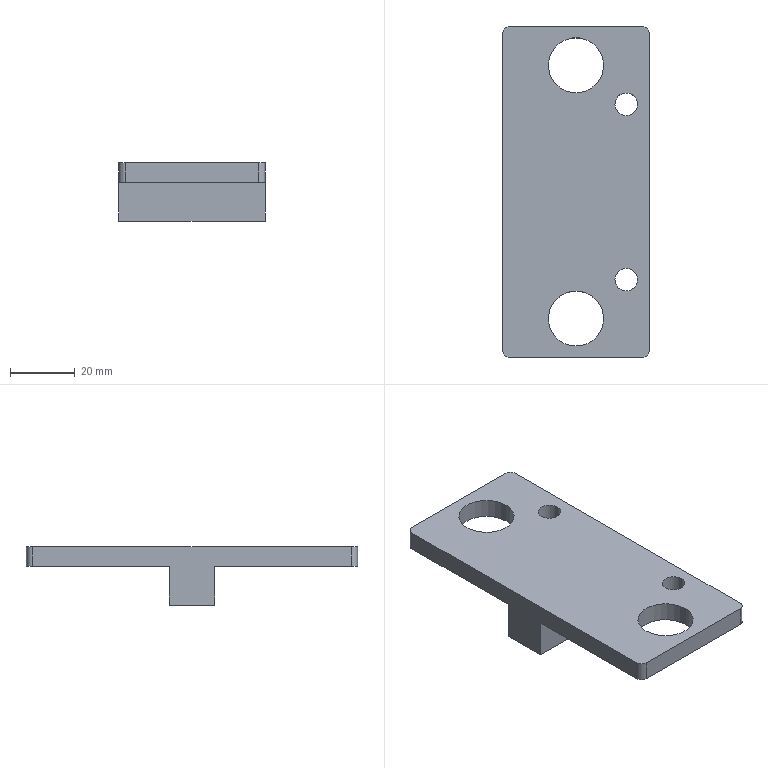Part | SolidWorks | features 3DProfileFeature 1, Extrusion 1, Fillet 1, HoleWzd 1, ICE 1, MirrorPattern 1 | 1 solid | 22 faces | box 45 x 102 x 18 mm | volume 31894 mm3 | cylinder 12 | plane 10 | commonest cylinder face diameters 4 x4 7 x4 17 x4
STEP:
#1=CARTESIAN_POINT('',(12.,-66.,0.));
#2=VERTEX_POINT('',#1);
#3=CARTESIAN_POINT('',(19.,-66.,0.));
#4=VERTEX_POINT('',#3);
#5=CARTESIAN_POINT('',(15.5,-66.,0.));
#6=DIRECTION('',(0.,0.,1.));
#7=DIRECTION('',(1.,0.,0.));
#8=AXIS2_PLACEMENT_3D('',#5,#6,#7);
#9=CIRCLE('',#8,3.5);
#10=EDGE_CURVE('',#2,#4,#9,.T.);
#11=ORIENTED_EDGE('',*,*,#10,.F.);
#12=CARTESIAN_POINT('',(12.,-66.,6.));
#13=VERTEX_POINT('',#12);
#14=CARTESIAN_POINT('',(12.,-66.,6.));
#15=DIRECTION('',(0.,0.,1.));
#16=VECTOR('',#15,1000.);
#17=LINE('',#14,#16);
#18=EDGE_CURVE('',#2,#13,#17,.T.);
#19=ORIENTED_EDGE('',*,*,#18,.T.);
#20=CARTESIAN_POINT('',(19.,-66.,6.));
#21=VERTEX_POINT('',#20);
#22=CARTESIAN_POINT('',(15.5,-66.,6.));
#23=DIRECTION('',(0.,0.,1.));
#24=DIRECTION('',(1.,0.,0.));
#25=AXIS2_PLACEMENT_3D('',#22,#23,#24);
#26=CIRCLE('',#25,3.5);
#27=EDGE_CURVE('',#13,#21,#26,.T.);
#28=ORIENTED_EDGE('',*,*,#27,.T.);
#29=CARTESIAN_POINT('',(19.,-66.,6.));
#30=DIRECTION('',(0.,0.,1.));
#31=VECTOR('',#30,1000.);
#32=LINE('',#29,#31);
#33=EDGE_CURVE('',#4,#21,#32,.T.);
#34=ORIENTED_EDGE('',*,*,#33,.F.);
#35=EDGE_LOOP('',(#11,#19,#28,#34));
#36=FACE_OUTER_BOUND('',#35,.T.);
#37=CARTESIAN_POINT('',(15.5,-66.,6.));
#38=DIRECTION('',(0.,0.,1.));
#39=DIRECTION('',(1.,0.,0.));
#40=AXIS2_PLACEMENT_3D('',#37,#38,#39);
#41=CYLINDRICAL_SURFACE('',#40,3.5);
#42=ADVANCED_FACE('',(#36),#41,.F.);
#43=CARTESIAN_POINT('',(8.5,-78.,6.));
#44=VERTEX_POINT('',#43);
#45=CARTESIAN_POINT('',(-8.5,-78.,6.));
#46=VERTEX_POINT('',#45);
#47=CARTESIAN_POINT('',(0.,-78.,6.));
#48=DIRECTION('',(0.,0.,-1.));
#49=DIRECTION('',(1.,0.,0.));
#50=AXIS2_PLACEMENT_3D('',#47,#48,#49);
#51=CIRCLE('',#50,8.5);
#52=EDGE_CURVE('',#44,#46,#51,.T.);
#53=ORIENTED_EDGE('',*,*,#52,.F.);
#54=CARTESIAN_POINT('',(8.5,-78.,0.));
#55=VERTEX_POINT('',#54);
#56=CARTESIAN_POINT('',(8.5,-78.,6.));
#57=DIRECTION('',(0.,0.,-1.));
#58=VECTOR('',#57,1000.);
#59=LINE('',#56,#58);
#60=EDGE_CURVE('',#44,#55,#59,.T.);
#61=ORIENTED_EDGE('',*,*,#60,.T.);
#62=CARTESIAN_POINT('',(-8.5,-78.,0.));
#63=VERTEX_POINT('',#62);
#64=CARTESIAN_POINT('',(0.,-78.,0.));
#65=DIRECTION('',(0.,0.,-1.));
#66=DIRECTION('',(1.,0.,0.));
#67=AXIS2_PLACEMENT_3D('',#64,#65,#66);
#68=CIRCLE('',#67,8.5);
#69=EDGE_CURVE('',#55,#63,#68,.T.);
#70=ORIENTED_EDGE('',*,*,#69,.T.);
#71=CARTESIAN_POINT('',(-8.5,-78.,6.));
#72=DIRECTION('',(0.,0.,-1.));
#73=VECTOR('',#72,1000.);
#74=LINE('',#71,#73);
#75=EDGE_CURVE('',#46,#63,#74,.T.);
#76=ORIENTED_EDGE('',*,*,#75,.F.);
#77=EDGE_LOOP('',(#53,#61,#70,#76));
#78=FACE_OUTER_BOUND('',#77,.T.);
#79=CARTESIAN_POINT('',(0.,-78.,6.));
#80=DIRECTION('',(0.,0.,-1.));
#81=DIRECTION('',(-1.,0.,0.));
#82=AXIS2_PLACEMENT_3D('',#79,#80,#81);
#83=CYLINDRICAL_SURFACE('',#82,8.5);
#84=ADVANCED_FACE('',(#78),#83,.F.);
#85=CARTESIAN_POINT('',(12.,-12.,0.));
#86=VERTEX_POINT('',#85);
#87=CARTESIAN_POINT('',(19.,-12.,0.));
#88=VERTEX_POINT('',#87);
#89=CARTESIAN_POINT('',(15.5,-12.,0.));
#90=DIRECTION('',(0.,0.,1.));
#91=DIRECTION('',(1.,0.,0.));
#92=AXIS2_PLACEMENT_3D('',#89,#90,#91);
#93=CIRCLE('',#92,3.5);
#94=EDGE_CURVE('',#86,#88,#93,.T.);
#95=ORIENTED_EDGE('',*,*,#94,.F.);
#96=CARTESIAN_POINT('',(12.,-12.,6.));
#97=VERTEX_POINT('',#96);
#98=CARTESIAN_POINT('',(12.,-12.,6.));
#99=DIRECTION('',(0.,0.,1.));
#100=VECTOR('',#99,1000.);
#101=LINE('',#98,#100);
#102=EDGE_CURVE('',#86,#97,#101,.T.);
#103=ORIENTED_EDGE('',*,*,#102,.T.);
#104=CARTESIAN_POINT('',(19.,-12.,6.));
#105=VERTEX_POINT('',#104);
#106=CARTESIAN_POINT('',(15.5,-12.,6.));
#107=DIRECTION('',(0.,0.,1.));
#108=DIRECTION('',(1.,0.,0.));
#109=AXIS2_PLACEMENT_3D('',#106,#107,#108);
#110=CIRCLE('',#109,3.5);
#111=EDGE_CURVE('',#97,#105,#110,.T.);
#112=ORIENTED_EDGE('',*,*,#111,.T.);
#113=CARTESIAN_POINT('',(19.,-12.,6.));
#114=DIRECTION('',(0.,0.,1.));
#115=VECTOR('',#114,1000.);
#116=LINE('',#113,#115);
#117=EDGE_CURVE('',#88,#105,#116,.T.);
#118=ORIENTED_EDGE('',*,*,#117,.F.);
#119=EDGE_LOOP('',(#95,#103,#112,#118));
#120=FACE_OUTER_BOUND('',#119,.T.);
#121=CARTESIAN_POINT('',(15.5,-12.,6.));
#122=DIRECTION('',(0.,0.,1.));
#123=DIRECTION('',(1.,0.,0.));
#124=AXIS2_PLACEMENT_3D('',#121,#122,#123);
#125=CYLINDRICAL_SURFACE('',#124,3.5);
#126=ADVANCED_FACE('',(#120),#125,.F.);
#127=CARTESIAN_POINT('',(-8.5,0.,6.));
#128=VERTEX_POINT('',#127);
#129=CARTESIAN_POINT('',(8.5,0.,6.));
#130=VERTEX_POINT('',#129);
#131=CARTESIAN_POINT('',(0.,0.,6.));
#132=DIRECTION('',(0.,0.,1.));
#133=DIRECTION('',(1.,0.,0.));
#134=AXIS2_PLACEMENT_3D('',#131,#132,#133);
#135=CIRCLE('',#134,8.5);
#136=EDGE_CURVE('',#128,#130,#135,.T.);
#137=ORIENTED_EDGE('',*,*,#136,.T.);
#138=CARTESIAN_POINT('',(8.5,0.,0.));
#139=VERTEX_POINT('',#138);
#140=CARTESIAN_POINT('',(8.5,0.,6.));
#141=DIRECTION('',(0.,0.,-1.));
#142=VECTOR('',#141,1000.);
#143=LINE('',#140,#142);
#144=EDGE_CURVE('',#130,#139,#143,.T.);
#145=ORIENTED_EDGE('',*,*,#144,.T.);
#146=CARTESIAN_POINT('',(-8.5,0.,0.));
#147=VERTEX_POINT('',#146);
#148=CARTESIAN_POINT('',(0.,0.,0.));
#149=DIRECTION('',(0.,0.,1.));
#150=DIRECTION('',(1.,0.,0.));
#151=AXIS2_PLACEMENT_3D('',#148,#149,#150);
#152=CIRCLE('',#151,8.5);
#153=EDGE_CURVE('',#147,#139,#152,.T.);
#154=ORIENTED_EDGE('',*,*,#153,.F.);
#155=CARTESIAN_POINT('',(-8.5,0.,6.));
#156=DIRECTION('',(0.,0.,-1.));
#157=VECTOR('',#156,1000.);
#158=LINE('',#155,#157);
#159=EDGE_CURVE('',#128,#147,#158,.T.);
#160=ORIENTED_EDGE('',*,*,#159,.F.);
#161=EDGE_LOOP('',(#137,#145,#154,#160));
#162=FACE_OUTER_BOUND('',#161,.T.);
#163=CARTESIAN_POINT('',(0.,0.,6.));
#164=DIRECTION('',(0.,0.,-1.));
#165=DIRECTION('',(-1.,0.,0.));
#166=AXIS2_PLACEMENT_3D('',#163,#164,#165);
#167=CYLINDRICAL_SURFACE('',#166,8.5);
#168=ADVANCED_FACE('',(#162),#167,.F.);
#169=CARTESIAN_POINT('',(-22.5,-46.,0.));
#170=VERTEX_POINT('',#169);
#171=CARTESIAN_POINT('',(22.5,-46.,0.));
#172=VERTEX_POINT('',#171);
#173=CARTESIAN_POINT('',(22.5,-46.,0.));
#174=DIRECTION('',(1.,0.,0.));
#175=VECTOR('',#174,1000.);
#176=LINE('',#173,#175);
#177=EDGE_CURVE('',#170,#172,#176,.T.);
#178=ORIENTED_EDGE('',*,*,#177,.F.);
#179=CARTESIAN_POINT('',(-22.5,-46.,-12.));
#180=VERTEX_POINT('',#179);
#181=CARTESIAN_POINT('',(-22.5,-46.,6.));
#182=DIRECTION('',(0.,0.,-1.));
#183=VECTOR('',#182,1000.);
#184=LINE('',#181,#183);
#185=EDGE_CURVE('',#170,#180,#184,.T.);
#186=ORIENTED_EDGE('',*,*,#185,.T.);
#187=CARTESIAN_POINT('',(22.5,-46.,-12.));
#188=VERTEX_POINT('',#187);
#189=CARTESIAN_POINT('',(22.5,-46.,-12.));
#190=DIRECTION('',(-1.,0.,0.));
#191=VECTOR('',#190,1000.);
#192=LINE('',#189,#191);
#193=EDGE_CURVE('',#188,#180,#192,.T.);
#194=ORIENTED_EDGE('',*,*,#193,.F.);
#195=CARTESIAN_POINT('',(22.5,-46.,6.));
#196=DIRECTION('',(0.,0.,-1.));
#197=VECTOR('',#196,1000.);
#198=LINE('',#195,#197);
#199=EDGE_CURVE('',#172,#188,#198,.T.);
#200=ORIENTED_EDGE('',*,*,#199,.F.);
#201=EDGE_LOOP('',(#178,#186,#194,#200));
#202=FACE_OUTER_BOUND('',#201,.T.);
#203=CARTESIAN_POINT('',(22.5,-46.,6.));
#204=DIRECTION('',(0.,1.,0.));
#205=DIRECTION('',(0.,0.,1.));
#206=AXIS2_PLACEMENT_3D('',#203,#204,#205);
#207=PLANE('',#206);
#208=ADVANCED_FACE('',(#202),#207,.F.);
#209=CARTESIAN_POINT('',(15.5,-12.,0.));
#210=DIRECTION('',(0.,0.,1.));
#211=DIRECTION('',(1.,0.,0.));
#212=AXIS2_PLACEMENT_3D('',#209,#210,#211);
#213=CIRCLE('',#212,3.5);
#214=EDGE_CURVE('',#88,#86,#213,.T.);
#215=ORIENTED_EDGE('',*,*,#214,.T.);
#216=ORIENTED_EDGE('',*,*,#94,.T.);
#217=EDGE_LOOP('',(#215,#216));
#218=FACE_BOUND('',#217,.T.);
#219=ORIENTED_EDGE('',*,*,#153,.T.);
#220=CARTESIAN_POINT('',(0.,0.,0.));
#221=DIRECTION('',(0.,0.,1.));
#222=DIRECTION('',(1.,0.,0.));
#223=AXIS2_PLACEMENT_3D('',#220,#221,#222);
#224=CIRCLE('',#223,8.5);
#225=EDGE_CURVE('',#139,#147,#224,.T.);
#226=ORIENTED_EDGE('',*,*,#225,.T.);
#227=EDGE_LOOP('',(#219,#226));
#228=FACE_BOUND('',#227,.T.);
#229=CARTESIAN_POINT('',(-22.5,10.,0.));
#230=VERTEX_POINT('',#229);
#231=CARTESIAN_POINT('',(-22.5,-32.,0.));
#232=VERTEX_POINT('',#231);
#233=CARTESIAN_POINT('',(-22.5,-46.,0.));
#234=DIRECTION('',(0.,-1.,0.));
#235=VECTOR('',#234,1000.);
#236=LINE('',#233,#235);
#237=EDGE_CURVE('',#230,#232,#236,.T.);
#238=ORIENTED_EDGE('',*,*,#237,.F.);
#239=CARTESIAN_POINT('',(-20.5,12.,0.));
#240=VERTEX_POINT('',#239);
#241=CARTESIAN_POINT('',(-20.5,10.,0.));
#242=DIRECTION('',(0.,0.,-1.));
#243=DIRECTION('',(1.,0.,0.));
#244=AXIS2_PLACEMENT_3D('',#241,#242,#243);
#245=CIRCLE('',#244,2.);
#246=EDGE_CURVE('',#230,#240,#245,.T.);
#247=ORIENTED_EDGE('',*,*,#246,.T.);
#248=CARTESIAN_POINT('',(20.5,12.,0.));
#249=VERTEX_POINT('',#248);
#250=CARTESIAN_POINT('',(22.5,12.,0.));
#251=DIRECTION('',(-1.,0.,0.));
#252=VECTOR('',#251,1000.);
#253=LINE('',#250,#252);
#254=EDGE_CURVE('',#249,#240,#253,.T.);
#255=ORIENTED_EDGE('',*,*,#254,.F.);
#256=CARTESIAN_POINT('',(22.5,10.,0.));
#257=VERTEX_POINT('',#256);
#258=CARTESIAN_POINT('',(20.5,10.,0.));
#259=DIRECTION('',(0.,0.,-1.));
#260=DIRECTION('',(1.,0.,0.));
#261=AXIS2_PLACEMENT_3D('',#258,#259,#260);
#262=CIRCLE('',#261,2.);
#263=EDGE_CURVE('',#249,#257,#262,.T.);
#264=ORIENTED_EDGE('',*,*,#263,.T.);
#265=CARTESIAN_POINT('',(22.5,-32.,0.));
#266=VERTEX_POINT('',#265);
#267=CARTESIAN_POINT('',(22.5,-46.,0.));
#268=DIRECTION('',(0.,1.,0.));
#269=VECTOR('',#268,1000.);
#270=LINE('',#267,#269);
#271=EDGE_CURVE('',#266,#257,#270,.T.);
#272=ORIENTED_EDGE('',*,*,#271,.F.);
#273=CARTESIAN_POINT('',(22.5,-32.,0.));
#274=DIRECTION('',(1.,0.,0.));
#275=VECTOR('',#274,1000.);
#276=LINE('',#273,#275);
#277=EDGE_CURVE('',#232,#266,#276,.T.);
#278=ORIENTED_EDGE('',*,*,#277,.F.);
#279=EDGE_LOOP('',(#238,#247,#255,#264,#272,#278));
#280=FACE_OUTER_BOUND('',#279,.T.);
#281=CARTESIAN_POINT('',(0.,0.,0.));
#282=DIRECTION('',(0.,0.,1.));
#283=DIRECTION('',(1.,0.,0.));
#284=AXIS2_PLACEMENT_3D('',#281,#282,#283);
#285=PLANE('',#284);
#286=ADVANCED_FACE('',(#218,#228,#280),#285,.F.);
#287=CARTESIAN_POINT('',(15.5,-66.,6.));
#288=DIRECTION('',(0.,0.,1.));
#289=DIRECTION('',(1.,0.,0.));
#290=AXIS2_PLACEMENT_3D('',#287,#288,#289);
#291=CIRCLE('',#290,3.5);
#292=EDGE_CURVE('',#21,#13,#291,.T.);
#293=ORIENTED_EDGE('',*,*,#292,.F.);
#294=ORIENTED_EDGE('',*,*,#27,.F.);
#295=EDGE_LOOP('',(#293,#294));
#296=FACE_BOUND('',#295,.T.);
#297=CARTESIAN_POINT('',(20.5,-90.,6.));
#298=VERTEX_POINT('',#297);
#299=CARTESIAN_POINT('',(-20.5,-90.,6.));
#300=VERTEX_POINT('',#299);
#301=CARTESIAN_POINT('',(22.5,-90.,6.));
#302=DIRECTION('',(-1.,0.,0.));
#303=VECTOR('',#302,1000.);
#304=LINE('',#301,#303);
#305=EDGE_CURVE('',#298,#300,#304,.T.);
#306=ORIENTED_EDGE('',*,*,#305,.F.);
#307=CARTESIAN_POINT('',(22.5,-88.,6.));
#308=VERTEX_POINT('',#307);
#309=CARTESIAN_POINT('',(20.5,-88.,6.));
#310=DIRECTION('',(0.,0.,1.));
#311=DIRECTION('',(1.,0.,0.));
#312=AXIS2_PLACEMENT_3D('',#309,#310,#311);
#313=CIRCLE('',#312,2.);
#314=EDGE_CURVE('',#298,#308,#313,.T.);
#315=ORIENTED_EDGE('',*,*,#314,.T.);
#316=CARTESIAN_POINT('',(22.5,10.,6.));
#317=VERTEX_POINT('',#316);
#318=CARTESIAN_POINT('',(22.5,-46.,6.));
#319=DIRECTION('',(0.,1.,0.));
#320=VECTOR('',#319,1000.);
#321=LINE('',#318,#320);
#322=EDGE_CURVE('',#308,#317,#321,.T.);
#323=ORIENTED_EDGE('',*,*,#322,.T.);
#324=CARTESIAN_POINT('',(20.5,12.,6.));
#325=VERTEX_POINT('',#324);
#326=CARTESIAN_POINT('',(20.5,10.,6.));
#327=DIRECTION('',(0.,0.,1.));
#328=DIRECTION('',(1.,0.,0.));
#329=AXIS2_PLACEMENT_3D('',#326,#327,#328);
#330=CIRCLE('',#329,2.);
#331=EDGE_CURVE('',#317,#325,#330,.T.);
#332=ORIENTED_EDGE('',*,*,#331,.T.);
#333=CARTESIAN_POINT('',(-20.5,12.,6.));
#334=VERTEX_POINT('',#333);
#335=CARTESIAN_POINT('',(22.5,12.,6.));
#336=DIRECTION('',(-1.,0.,0.));
#337=VECTOR('',#336,1000.);
#338=LINE('',#335,#337);
#339=EDGE_CURVE('',#325,#334,#338,.T.);
#340=ORIENTED_EDGE('',*,*,#339,.T.);
#341=CARTESIAN_POINT('',(-22.5,10.,6.));
#342=VERTEX_POINT('',#341);
#343=CARTESIAN_POINT('',(-20.5,10.,6.));
#344=DIRECTION('',(0.,0.,1.));
#345=DIRECTION('',(1.,0.,0.));
#346=AXIS2_PLACEMENT_3D('',#343,#344,#345);
#347=CIRCLE('',#346,2.);
#348=EDGE_CURVE('',#334,#342,#347,.T.);
#349=ORIENTED_EDGE('',*,*,#348,.T.);
#350=CARTESIAN_POINT('',(-22.5,-88.,6.));
#351=VERTEX_POINT('',#350);
#352=CARTESIAN_POINT('',(-22.5,-46.,6.));
#353=DIRECTION('',(0.,-1.,0.));
#354=VECTOR('',#353,1000.);
#355=LINE('',#352,#354);
#356=EDGE_CURVE('',#342,#351,#355,.T.);
#357=ORIENTED_EDGE('',*,*,#356,.T.);
#358=CARTESIAN_POINT('',(-20.5,-88.,6.));
#359=DIRECTION('',(0.,0.,1.));
#360=DIRECTION('',(1.,0.,0.));
#361=AXIS2_PLACEMENT_3D('',#358,#359,#360);
#362=CIRCLE('',#361,2.);
#363=EDGE_CURVE('',#351,#300,#362,.T.);
#364=ORIENTED_EDGE('',*,*,#363,.T.);
#365=EDGE_LOOP('',(#306,#315,#323,#332,#340,#349,#357,#364));
#366=FACE_OUTER_BOUND('',#365,.T.);
#367=CARTESIAN_POINT('',(15.5,-12.,6.));
#368=DIRECTION('',(0.,0.,1.));
#369=DIRECTION('',(1.,0.,0.));
#370=AXIS2_PLACEMENT_3D('',#367,#368,#369);
#371=CIRCLE('',#370,3.5);
#372=EDGE_CURVE('',#105,#97,#371,.T.);
#373=ORIENTED_EDGE('',*,*,#372,.F.);
#374=ORIENTED_EDGE('',*,*,#111,.F.);
#375=EDGE_LOOP('',(#373,#374));
#376=FACE_BOUND('',#375,.T.);
#377=ORIENTED_EDGE('',*,*,#136,.F.);
#378=CARTESIAN_POINT('',(0.,0.,6.));
#379=DIRECTION('',(0.,0.,1.));
#380=DIRECTION('',(1.,0.,0.));
#381=AXIS2_PLACEMENT_3D('',#378,#379,#380);
#382=CIRCLE('',#381,8.5);
#383=EDGE_CURVE('',#130,#128,#382,.T.);
#384=ORIENTED_EDGE('',*,*,#383,.F.);
#385=EDGE_LOOP('',(#377,#384));
#386=FACE_BOUND('',#385,.T.);
#387=CARTESIAN_POINT('',(0.,-78.,6.));
#388=DIRECTION('',(0.,0.,-1.));
#389=DIRECTION('',(1.,0.,0.));
#390=AXIS2_PLACEMENT_3D('',#387,#388,#389);
#391=CIRCLE('',#390,8.5);
#392=EDGE_CURVE('',#46,#44,#391,.T.);
#393=ORIENTED_EDGE('',*,*,#392,.T.);
#394=ORIENTED_EDGE('',*,*,#52,.T.);
#395=EDGE_LOOP('',(#393,#394));
#396=FACE_BOUND('',#395,.T.);
#397=CARTESIAN_POINT('',(0.,0.,6.));
#398=DIRECTION('',(0.,0.,1.));
#399=DIRECTION('',(1.,0.,0.));
#400=AXIS2_PLACEMENT_3D('',#397,#398,#399);
#401=PLANE('',#400);
#402=ADVANCED_FACE('',(#296,#366,#376,#386,#396),#401,.T.);
#403=CARTESIAN_POINT('',(-22.5,-88.,0.));
#404=VERTEX_POINT('',#403);
#405=CARTESIAN_POINT('',(-22.5,-32.,0.));
#406=DIRECTION('',(0.,1.,0.));
#407=VECTOR('',#406,1000.);
#408=LINE('',#405,#407);
#409=EDGE_CURVE('',#404,#170,#408,.T.);
#410=ORIENTED_EDGE('',*,*,#409,.F.);
#411=CARTESIAN_POINT('',(-22.5,-88.,6.));
#412=DIRECTION('',(0.,0.,1.));
#413=VECTOR('',#412,1000.);
#414=LINE('',#411,#413);
#415=EDGE_CURVE('',#404,#351,#414,.T.);
#416=ORIENTED_EDGE('',*,*,#415,.T.);
#417=ORIENTED_EDGE('',*,*,#356,.F.);
#418=CARTESIAN_POINT('',(-22.5,10.,6.));
#419=DIRECTION('',(0.,0.,-1.));
#420=VECTOR('',#419,1000.);
#421=LINE('',#418,#420);
#422=EDGE_CURVE('',#342,#230,#421,.T.);
#423=ORIENTED_EDGE('',*,*,#422,.T.);
#424=ORIENTED_EDGE('',*,*,#237,.T.);
#425=CARTESIAN_POINT('',(-22.5,-32.,-12.));
#426=VERTEX_POINT('',#425);
#427=CARTESIAN_POINT('',(-22.5,-32.,-12.));
#428=DIRECTION('',(0.,0.,1.));
#429=VECTOR('',#428,1000.);
#430=LINE('',#427,#429);
#431=EDGE_CURVE('',#426,#232,#430,.T.);
#432=ORIENTED_EDGE('',*,*,#431,.F.);
#433=CARTESIAN_POINT('',(-22.5,-46.,-12.));
#434=DIRECTION('',(0.,1.,0.));
#435=VECTOR('',#434,1000.);
#436=LINE('',#433,#435);
#437=EDGE_CURVE('',#180,#426,#436,.T.);
#438=ORIENTED_EDGE('',*,*,#437,.F.);
#439=ORIENTED_EDGE('',*,*,#185,.F.);
#440=EDGE_LOOP('',(#410,#416,#417,#423,#424,#432,#438,#439));
#441=FACE_OUTER_BOUND('',#440,.T.);
#442=CARTESIAN_POINT('',(-22.5,-46.,6.));
#443=DIRECTION('',(1.,0.,0.));
#444=DIRECTION('',(0.,0.,-1.));
#445=AXIS2_PLACEMENT_3D('',#442,#443,#444);
#446=PLANE('',#445);
#447=ADVANCED_FACE('',(#441),#446,.F.);
#448=ORIENTED_EDGE('',*,*,#322,.F.);
#449=CARTESIAN_POINT('',(22.5,-88.,0.));
#450=VERTEX_POINT('',#449);
#451=CARTESIAN_POINT('',(22.5,-88.,0.));
#452=DIRECTION('',(0.,0.,-1.));
#453=VECTOR('',#452,1000.);
#454=LINE('',#451,#453);
#455=EDGE_CURVE('',#308,#450,#454,.T.);
#456=ORIENTED_EDGE('',*,*,#455,.T.);
#457=CARTESIAN_POINT('',(22.5,-32.,0.));
#458=DIRECTION('',(0.,-1.,0.));
#459=VECTOR('',#458,1000.);
#460=LINE('',#457,#459);
#461=EDGE_CURVE('',#172,#450,#460,.T.);
#462=ORIENTED_EDGE('',*,*,#461,.F.);
#463=ORIENTED_EDGE('',*,*,#199,.T.);
#464=CARTESIAN_POINT('',(22.5,-32.,-12.));
#465=VERTEX_POINT('',#464);
#466=CARTESIAN_POINT('',(22.5,-46.,-12.));
#467=DIRECTION('',(0.,-1.,0.));
#468=VECTOR('',#467,1000.);
#469=LINE('',#466,#468);
#470=EDGE_CURVE('',#465,#188,#469,.T.);
#471=ORIENTED_EDGE('',*,*,#470,.F.);
#472=CARTESIAN_POINT('',(22.5,-32.,-12.));
#473=DIRECTION('',(0.,0.,1.));
#474=VECTOR('',#473,1000.);
#475=LINE('',#472,#474);
#476=EDGE_CURVE('',#465,#266,#475,.T.);
#477=ORIENTED_EDGE('',*,*,#476,.T.);
#478=ORIENTED_EDGE('',*,*,#271,.T.);
#479=CARTESIAN_POINT('',(22.5,10.,6.));
#480=DIRECTION('',(0.,0.,1.));
#481=VECTOR('',#480,1000.);
#482=LINE('',#479,#481);
#483=EDGE_CURVE('',#257,#317,#482,.T.);
#484=ORIENTED_EDGE('',*,*,#483,.T.);
#485=EDGE_LOOP('',(#448,#456,#462,#463,#471,#477,#478,#484));
#486=FACE_OUTER_BOUND('',#485,.T.);
#487=CARTESIAN_POINT('',(22.5,-46.,6.));
#488=DIRECTION('',(-1.,0.,0.));
#489=DIRECTION('',(0.,0.,1.));
#490=AXIS2_PLACEMENT_3D('',#487,#488,#489);
#491=PLANE('',#490);
#492=ADVANCED_FACE('',(#486),#491,.F.);
#493=ORIENTED_EDGE('',*,*,#254,.T.);
#494=CARTESIAN_POINT('',(-20.5,12.,6.));
#495=DIRECTION('',(0.,0.,1.));
#496=VECTOR('',#495,1000.);
#497=LINE('',#494,#496);
#498=EDGE_CURVE('',#240,#334,#497,.T.);
#499=ORIENTED_EDGE('',*,*,#498,.T.);
#500=ORIENTED_EDGE('',*,*,#339,.F.);
#501=CARTESIAN_POINT('',(20.5,12.,6.));
#502=DIRECTION('',(0.,0.,-1.));
#503=VECTOR('',#502,1000.);
#504=LINE('',#501,#503);
#505=EDGE_CURVE('',#325,#249,#504,.T.);
#506=ORIENTED_EDGE('',*,*,#505,.T.);
#507=EDGE_LOOP('',(#493,#499,#500,#506));
#508=FACE_OUTER_BOUND('',#507,.T.);
#509=CARTESIAN_POINT('',(22.5,12.,6.));
#510=DIRECTION('',(0.,-1.,0.));
#511=DIRECTION('',(1.,0.,0.));
#512=AXIS2_PLACEMENT_3D('',#509,#510,#511);
#513=PLANE('',#512);
#514=ADVANCED_FACE('',(#508),#513,.F.);
#515=ORIENTED_EDGE('',*,*,#144,.F.);
#516=ORIENTED_EDGE('',*,*,#383,.T.);
#517=ORIENTED_EDGE('',*,*,#159,.T.);
#518=ORIENTED_EDGE('',*,*,#225,.F.);
#519=EDGE_LOOP('',(#515,#516,#517,#518));
#520=FACE_OUTER_BOUND('',#519,.T.);
#521=CARTESIAN_POINT('',(0.,0.,6.));
#522=DIRECTION('',(0.,0.,-1.));
#523=DIRECTION('',(-1.,0.,0.));
#524=AXIS2_PLACEMENT_3D('',#521,#522,#523);
#525=CYLINDRICAL_SURFACE('',#524,8.5);
#526=ADVANCED_FACE('',(#520),#525,.F.);
#527=ORIENTED_EDGE('',*,*,#277,.T.);
#528=ORIENTED_EDGE('',*,*,#476,.F.);
#529=CARTESIAN_POINT('',(22.5,-32.,-12.));
#530=DIRECTION('',(1.,0.,0.));
#531=VECTOR('',#530,1000.);
#532=LINE('',#529,#531);
#533=EDGE_CURVE('',#426,#465,#532,.T.);
#534=ORIENTED_EDGE('',*,*,#533,.F.);
#535=ORIENTED_EDGE('',*,*,#431,.T.);
#536=EDGE_LOOP('',(#527,#528,#534,#535));
#537=FACE_OUTER_BOUND('',#536,.T.);
#538=CARTESIAN_POINT('',(22.5,-32.,-12.));
#539=DIRECTION('',(0.,-1.,0.));
#540=DIRECTION('',(0.,0.,-1.));
#541=AXIS2_PLACEMENT_3D('',#538,#539,#540);
#542=PLANE('',#541);
#543=ADVANCED_FACE('',(#537),#542,.F.);
#544=ORIENTED_EDGE('',*,*,#470,.T.);
#545=ORIENTED_EDGE('',*,*,#193,.T.);
#546=ORIENTED_EDGE('',*,*,#437,.T.);
#547=ORIENTED_EDGE('',*,*,#533,.T.);
#548=EDGE_LOOP('',(#544,#545,#546,#547));
#549=FACE_OUTER_BOUND('',#548,.T.);
#550=CARTESIAN_POINT('',(0.,0.,-12.));
#551=DIRECTION('',(0.,0.,1.));
#552=DIRECTION('',(1.,0.,0.));
#553=AXIS2_PLACEMENT_3D('',#550,#551,#552);
#554=PLANE('',#553);
#555=ADVANCED_FACE('',(#549),#554,.F.);
#556=ORIENTED_EDGE('',*,*,#102,.F.);
#557=ORIENTED_EDGE('',*,*,#214,.F.);
#558=ORIENTED_EDGE('',*,*,#117,.T.);
#559=ORIENTED_EDGE('',*,*,#372,.T.);
#560=EDGE_LOOP('',(#556,#557,#558,#559));
#561=FACE_OUTER_BOUND('',#560,.T.);
#562=CARTESIAN_POINT('',(15.5,-12.,6.));
#563=DIRECTION('',(0.,0.,1.));
#564=DIRECTION('',(1.,0.,0.));
#565=AXIS2_PLACEMENT_3D('',#562,#563,#564);
#566=CYLINDRICAL_SURFACE('',#565,3.5);
#567=ADVANCED_FACE('',(#561),#566,.F.);
#568=CARTESIAN_POINT('',(15.5,-66.,0.));
#569=DIRECTION('',(0.,0.,1.));
#570=DIRECTION('',(1.,0.,0.));
#571=AXIS2_PLACEMENT_3D('',#568,#569,#570);
#572=CIRCLE('',#571,3.5);
#573=EDGE_CURVE('',#4,#2,#572,.T.);
#574=ORIENTED_EDGE('',*,*,#573,.T.);
#575=ORIENTED_EDGE('',*,*,#10,.T.);
#576=EDGE_LOOP('',(#574,#575));
#577=FACE_BOUND('',#576,.T.);
#578=CARTESIAN_POINT('',(0.,-78.,0.));
#579=DIRECTION('',(0.,0.,-1.));
#580=DIRECTION('',(1.,0.,0.));
#581=AXIS2_PLACEMENT_3D('',#578,#579,#580);
#582=CIRCLE('',#581,8.5);
#583=EDGE_CURVE('',#63,#55,#582,.T.);
#584=ORIENTED_EDGE('',*,*,#583,.F.);
#585=ORIENTED_EDGE('',*,*,#69,.F.);
#586=EDGE_LOOP('',(#584,#585));
#587=FACE_BOUND('',#586,.T.);
#588=ORIENTED_EDGE('',*,*,#461,.T.);
#589=CARTESIAN_POINT('',(20.5,-90.,0.));
#590=VERTEX_POINT('',#589);
#591=CARTESIAN_POINT('',(20.5,-88.,0.));
#592=DIRECTION('',(0.,0.,-1.));
#593=DIRECTION('',(1.,0.,0.));
#594=AXIS2_PLACEMENT_3D('',#591,#592,#593);
#595=CIRCLE('',#594,2.);
#596=EDGE_CURVE('',#450,#590,#595,.T.);
#597=ORIENTED_EDGE('',*,*,#596,.T.);
#598=CARTESIAN_POINT('',(-20.5,-90.,0.));
#599=VERTEX_POINT('',#598);
#600=CARTESIAN_POINT('',(22.5,-90.,0.));
#601=DIRECTION('',(-1.,0.,0.));
#602=VECTOR('',#601,1000.);
#603=LINE('',#600,#602);
#604=EDGE_CURVE('',#590,#599,#603,.T.);
#605=ORIENTED_EDGE('',*,*,#604,.T.);
#606=CARTESIAN_POINT('',(-20.5,-88.,0.));
#607=DIRECTION('',(0.,0.,-1.));
#608=DIRECTION('',(1.,0.,0.));
#609=AXIS2_PLACEMENT_3D('',#606,#607,#608);
#610=CIRCLE('',#609,2.);
#611=EDGE_CURVE('',#599,#404,#610,.T.);
#612=ORIENTED_EDGE('',*,*,#611,.T.);
#613=ORIENTED_EDGE('',*,*,#409,.T.);
#614=ORIENTED_EDGE('',*,*,#177,.T.);
#615=EDGE_LOOP('',(#588,#597,#605,#612,#613,#614));
#616=FACE_OUTER_BOUND('',#615,.T.);
#617=CARTESIAN_POINT('',(0.,-78.,0.));
#618=DIRECTION('',(0.,0.,1.));
#619=DIRECTION('',(1.,0.,0.));
#620=AXIS2_PLACEMENT_3D('',#617,#618,#619);
#621=PLANE('',#620);
#622=ADVANCED_FACE('',(#577,#587,#616),#621,.F.);
#623=ORIENTED_EDGE('',*,*,#604,.F.);
#624=CARTESIAN_POINT('',(20.5,-90.,6.));
#625=DIRECTION('',(0.,0.,1.));
#626=VECTOR('',#625,1000.);
#627=LINE('',#624,#626);
#628=EDGE_CURVE('',#590,#298,#627,.T.);
#629=ORIENTED_EDGE('',*,*,#628,.T.);
#630=ORIENTED_EDGE('',*,*,#305,.T.);
#631=CARTESIAN_POINT('',(-20.5,-90.,0.));
#632=DIRECTION('',(0.,0.,-1.));
#633=VECTOR('',#632,1000.);
#634=LINE('',#631,#633);
#635=EDGE_CURVE('',#300,#599,#634,.T.);
#636=ORIENTED_EDGE('',*,*,#635,.T.);
#637=EDGE_LOOP('',(#623,#629,#630,#636));
#638=FACE_OUTER_BOUND('',#637,.T.);
#639=CARTESIAN_POINT('',(22.5,-90.,6.));
#640=DIRECTION('',(0.,-1.,0.));
#641=DIRECTION('',(1.,0.,0.));
#642=AXIS2_PLACEMENT_3D('',#639,#640,#641);
#643=PLANE('',#642);
#644=ADVANCED_FACE('',(#638),#643,.T.);
#645=ORIENTED_EDGE('',*,*,#60,.F.);
#646=ORIENTED_EDGE('',*,*,#392,.F.);
#647=ORIENTED_EDGE('',*,*,#75,.T.);
#648=ORIENTED_EDGE('',*,*,#583,.T.);
#649=EDGE_LOOP('',(#645,#646,#647,#648));
#650=FACE_OUTER_BOUND('',#649,.T.);
#651=CARTESIAN_POINT('',(0.,-78.,6.));
#652=DIRECTION('',(0.,0.,-1.));
#653=DIRECTION('',(-1.,0.,0.));
#654=AXIS2_PLACEMENT_3D('',#651,#652,#653);
#655=CYLINDRICAL_SURFACE('',#654,8.5);
#656=ADVANCED_FACE('',(#650),#655,.F.);
#657=ORIENTED_EDGE('',*,*,#18,.F.);
#658=ORIENTED_EDGE('',*,*,#573,.F.);
#659=ORIENTED_EDGE('',*,*,#33,.T.);
#660=ORIENTED_EDGE('',*,*,#292,.T.);
#661=EDGE_LOOP('',(#657,#658,#659,#660));
#662=FACE_OUTER_BOUND('',#661,.T.);
#663=CARTESIAN_POINT('',(15.5,-66.,6.));
#664=DIRECTION('',(0.,0.,1.));
#665=DIRECTION('',(1.,0.,0.));
#666=AXIS2_PLACEMENT_3D('',#663,#664,#665);
#667=CYLINDRICAL_SURFACE('',#666,3.5);
#668=ADVANCED_FACE('',(#662),#667,.F.);
#669=ORIENTED_EDGE('',*,*,#314,.F.);
#670=ORIENTED_EDGE('',*,*,#628,.F.);
#671=ORIENTED_EDGE('',*,*,#596,.F.);
#672=ORIENTED_EDGE('',*,*,#455,.F.);
#673=EDGE_LOOP('',(#669,#670,#671,#672));
#674=FACE_OUTER_BOUND('',#673,.T.);
#675=CARTESIAN_POINT('',(20.5,-88.,6.));
#676=DIRECTION('',(0.,0.,1.));
#677=DIRECTION('',(1.,0.,0.));
#678=AXIS2_PLACEMENT_3D('',#675,#676,#677);
#679=CYLINDRICAL_SURFACE('',#678,2.);
#680=ADVANCED_FACE('',(#674),#679,.T.);
#681=ORIENTED_EDGE('',*,*,#363,.F.);
#682=ORIENTED_EDGE('',*,*,#415,.F.);
#683=ORIENTED_EDGE('',*,*,#611,.F.);
#684=ORIENTED_EDGE('',*,*,#635,.F.);
#685=EDGE_LOOP('',(#681,#682,#683,#684));
#686=FACE_OUTER_BOUND('',#685,.T.);
#687=CARTESIAN_POINT('',(-20.5,-88.,6.));
#688=DIRECTION('',(0.,0.,1.));
#689=DIRECTION('',(1.,0.,0.));
#690=AXIS2_PLACEMENT_3D('',#687,#688,#689);
#691=CYLINDRICAL_SURFACE('',#690,2.);
#692=ADVANCED_FACE('',(#686),#691,.T.);
#693=ORIENTED_EDGE('',*,*,#348,.F.);
#694=ORIENTED_EDGE('',*,*,#498,.F.);
#695=ORIENTED_EDGE('',*,*,#246,.F.);
#696=ORIENTED_EDGE('',*,*,#422,.F.);
#697=EDGE_LOOP('',(#693,#694,#695,#696));
#698=FACE_OUTER_BOUND('',#697,.T.);
#699=CARTESIAN_POINT('',(-20.5,10.,6.));
#700=DIRECTION('',(0.,0.,-1.));
#701=DIRECTION('',(-1.,0.,0.));
#702=AXIS2_PLACEMENT_3D('',#699,#700,#701);
#703=CYLINDRICAL_SURFACE('',#702,2.);
#704=ADVANCED_FACE('',(#698),#703,.T.);
#705=ORIENTED_EDGE('',*,*,#331,.F.);
#706=ORIENTED_EDGE('',*,*,#483,.F.);
#707=ORIENTED_EDGE('',*,*,#263,.F.);
#708=ORIENTED_EDGE('',*,*,#505,.F.);
#709=EDGE_LOOP('',(#705,#706,#707,#708));
#710=FACE_OUTER_BOUND('',#709,.T.);
#711=CARTESIAN_POINT('',(20.5,10.,6.));
#712=DIRECTION('',(0.,0.,-1.));
#713=DIRECTION('',(-1.,0.,0.));
#714=AXIS2_PLACEMENT_3D('',#711,#712,#713);
#715=CYLINDRICAL_SURFACE('',#714,2.);
#716=ADVANCED_FACE('',(#710),#715,.T.);
#717=CLOSED_SHELL('',(#42,#84,#126,#168,#208,#286,#402,#447,#492,#514,#526,#543,#555,#567,#622,#644,#656,#668,#680,#692,#704,#716));
#718=MANIFOLD_SOLID_BREP('',#717);
#719=CARTESIAN_POINT('',(0.,0.,0.));
#720=DIRECTION('',(0.,0.,1.));
#721=DIRECTION('',(1.,0.,0.));
#722=AXIS2_PLACEMENT_3D('',#719,#720,#721);
#723=(LENGTH_UNIT()NAMED_UNIT(*)SI_UNIT(.MILLI.,.METRE.));
#724=UNCERTAINTY_MEASURE_WITH_UNIT(LENGTH_MEASURE(0.00001),#723,'','');
#725=(NAMED_UNIT(*)PLANE_ANGLE_UNIT()SI_UNIT($,.RADIAN.));
#726=(NAMED_UNIT(*)SI_UNIT($,.STERADIAN.)SOLID_ANGLE_UNIT());
#727=(GEOMETRIC_REPRESENTATION_CONTEXT(3)GLOBAL_UNCERTAINTY_ASSIGNED_CONTEXT((#724))GLOBAL_UNIT_ASSIGNED_CONTEXT((#723,#725,#726))REPRESENTATION_CONTEXT('',''));
#728=ADVANCED_BREP_SHAPE_REPRESENTATION('',(#718,#722),#727);